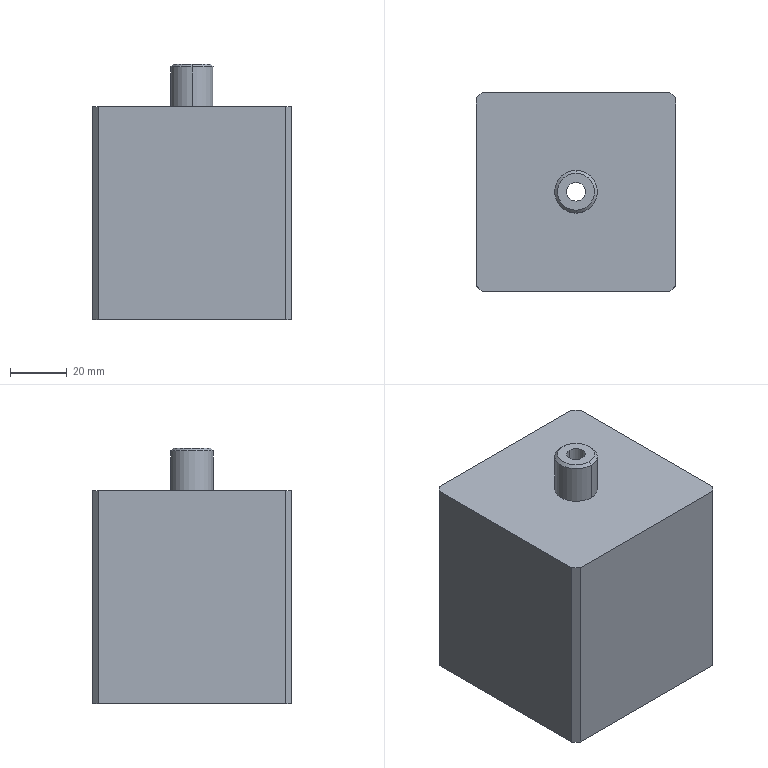NC program | NX | posted with a generic post | part box 70 x 70 x 90 mm
Lines 107 to 966 of 10206:
(ZLEVEL_PROFILE_COPY_1_COPY , TOOL : D16)
N212 T22 M6
N214 G54
N216 G17 G0 G90 X-6.657 Y-6.984 S7500 M3
N218 G43 Z30. H22
N220 Z1.4
N222 G94 G1 X-5.215 Y-7.622 Z1.317 F1000.
N224 X-2.644 Y-8.278 Z1.178
N226 X0. Y-8.499 Z1.039
N228 X2.644 Y-8.278 Z0.9
N230 X5.215 Y-7.622 Z0.761
N232 X7.642 Y-6.548 Z0.622
N234 X8.469 Y-6.028 Z0.571
N236 Y6.028 Z-0.061
N238 X7.642 Y6.548 Z-0.112
N240 X5.215 Y7.622 Z-0.251
N242 X2.644 Y8.278 Z-0.39
N244 X0. Y8.499 Z-0.529
N246 X-2.644 Y8.278 Z-0.668
N248 X-5.215 Y7.622 Z-0.808
N250 X-7.642 Y6.548 Z-0.947
N252 X-8.469 Y6.028 Z-0.998
N254 Y-6.028 F2500.
N256 G3 X8.469 Y-6.028 R15.91
N258 G1 Y6.028
N260 G3 X-8.469 Y6.028 R15.91
N262 G1 X-8.461 Y5.368 Z-1.013
N264 X-8.452 Y4.709 Z-1.028
N266 X-8.444 Y4.049 Z-1.043
N268 X-8.436 Y3.389 Z-1.058
N270 X-8.428 Y2.73 Z-1.073
N272 X-8.42 Y2.07 Z-1.089
N274 X-8.412 Y1.411 Z-1.104
N276 X-8.405 Y0.751 Z-1.119
N278 X-8.397 Y0.092 Z-1.134
N280 X-8.39 Y-0.568 Z-1.149
N282 X-8.383 Y-1.228 Z-1.164
N284 X-8.376 Y-1.887 Z-1.179
N286 X-8.369 Y-2.547 Z-1.194
N288 X-8.363 Y-3.206 Z-1.209
N290 X-8.356 Y-3.866 Z-1.225
N292 X-8.35 Y-4.525 Z-1.24
N294 X-8.344 Y-5.185 Z-1.255
N296 X-8.338 Y-5.845 Z-1.27
N298 X-8.337 Y-5.954 Z-1.273
N300 X-7.992 Y-6.158 Z-1.283
N302 X-7.42 Y-6.472 Z-1.3
N304 X-6.834 Y-6.762 Z-1.315
N306 X-6.238 Y-7.028 Z-1.33
N308 X-5.631 Y-7.269 Z-1.346
N310 X-5.014 Y-7.485 Z-1.361
N312 X-4.39 Y-7.675 Z-1.376
N314 X-3.759 Y-7.84 Z-1.391
N316 X-3.121 Y-7.977 Z-1.406
N318 X-2.479 Y-8.089 Z-1.421
N320 X-1.833 Y-8.174 Z-1.436
N322 X-1.184 Y-8.232 Z-1.451
N324 X-0.533 Y-8.263 Z-1.466
N326 X0.118 Y-8.268 Z-1.482
N328 X0.769 Y-8.246 Z-1.497
N330 X1.418 Y-8.196 Z-1.512
N332 X2.065 Y-8.12 Z-1.527
N334 X2.707 Y-8.018 Z-1.542
N336 X3.345 Y-7.889 Z-1.557
N338 X3.976 Y-7.734 Z-1.572
N340 X4.601 Y-7.553 Z-1.587
N342 X5.217 Y-7.346 Z-1.603
N344 X5.824 Y-7.115 Z-1.618
N346 X6.422 Y-6.858 Z-1.633
N348 X7.403 Y-6.371 Z-1.658
N350 X7.581 Y-6.272 Z-1.663
N352 X8.203 Y-5.906 Z-1.684
N354 X8.224 Y-5.605 Z-1.693
N356 X8.221 Y-4.945 Z-1.708
N358 X8.219 Y-4.285 Z-1.723
N360 X8.217 Y-3.626 Z-1.739
N362 X8.215 Y-2.966 Z-1.754
N364 X8.213 Y-2.307 Z-1.769
N366 X8.212 Y-1.647 Z-1.784
N368 X8.21 Y-0.988 Z-1.799
N370 X8.209 Y-0.328 Z-1.814
N372 X8.207 Y0.331 Z-1.829
N374 X8.206 Y0.991 Z-1.844
N376 X8.205 Y1.651 Z-1.86
N378 X8.204 Y2.31 Z-1.875
N380 X8.203 Y2.97 Z-1.89
N382 X8.202 Y3.629 Z-1.905
N384 Y4.289 Z-1.92
N386 X8.201 Y4.948 Z-1.935
N388 X8.197 Y5.881 Z-1.963
N390 X7.564 Y6.249 Z-1.98
N392 X6.991 Y6.551 Z-1.996
N394 G3 X-8.203 Y5.876 R15.64
N396 G1 X-8.2 Y5.216 Z-2.011
N398 Y4.557 Z-2.026
N400 Y-4.676 Z-2.237
N402 X-8.195 Y-5.881 Z-2.265
N404 X-8.1 Y-5.939 Z-2.268
N406 X-7.529 Y-6.269 Z-2.283
N408 X-6.944 Y-6.574 Z-2.298
N410 X-6.347 Y-6.854 Z-2.313
N412 X-5.739 Y-7.109 Z-2.328
N414 X-5.12 Y-7.338 Z-2.343
N416 X-4.493 Y-7.541 Z-2.358
N418 X-3.857 Y-7.717 Z-2.374
N420 X-3.215 Y-7.866 Z-2.389
N422 X-2.567 Y-7.988 Z-2.404
N424 X-1.914 Y-8.082 Z-2.419
N426 X-1.258 Y-8.149 Z-2.434
N428 X-0.6 Y-8.188 Z-2.449
N430 X0.06 Y-8.2 Z-2.464
N432 X0.719 Y-8.183 Z-2.479
N434 X1.377 Y-8.139 Z-2.494
N436 X2.032 Y-8.067 Z-2.51
N438 X2.684 Y-7.968 Z-2.525
N440 X3.332 Y-7.841 Z-2.54
N442 X3.973 Y-7.687 Z-2.555
N444 X4.607 Y-7.506 Z-2.57
N446 X5.233 Y-7.299 Z-2.585
N448 X5.85 Y-7.065 Z-2.6
N450 X6.456 Y-6.805 Z-2.615
N452 X7.051 Y-6.521 Z-2.631
N454 X8.126 Y-5.924 Z-2.659
N456 X8.2 Y-5.876 Z-2.661
N458 Y-5.217 Z-2.676
N460 Y4.676 Z-2.903
N462 X8.196 Y5.882 Z-2.93
N464 X8.101 Y5.938 Z-2.933
N466 X7.53 Y6.268 Z-2.948
N468 X6.946 Y6.573 Z-2.963
N470 X6.349 Y6.853 Z-2.978
N472 X5.741 Y7.108 Z-2.993
N474 G3 X-8.2 Y5.878 R15.64
N476 G1 Y5.876
N478 Y-4.676 Z-3.235
N480 X-8.195 Y-5.881 Z-3.263
N482 X-8.1 Y-5.939 Z-3.266
N484 X-7.529 Y-6.269 Z-3.281
N486 X-6.944 Y-6.574 Z-3.296
N488 X-6.347 Y-6.854 Z-3.311
N490 X-5.739 Y-7.109 Z-3.326
N492 X-5.12 Y-7.338 Z-3.341
N494 X-4.493 Y-7.541 Z-3.356
N496 X-3.857 Y-7.717 Z-3.371
N498 X-3.215 Y-7.866 Z-3.386
N500 X-2.567 Y-7.988 Z-3.402
N502 X-1.914 Y-8.082 Z-3.417
N504 X-1.258 Y-8.149 Z-3.432
N506 X-0.6 Y-8.188 Z-3.447
N508 X0.06 Y-8.2 Z-3.462
N510 X0.719 Y-8.183 Z-3.477
N512 X1.377 Y-8.139 Z-3.492
N514 X2.032 Y-8.067 Z-3.507
N516 X2.684 Y-7.968 Z-3.523
N518 X3.332 Y-7.841 Z-3.538
N520 X3.973 Y-7.687 Z-3.553
N522 X4.607 Y-7.506 Z-3.568
N524 X5.233 Y-7.299 Z-3.583
N526 X5.85 Y-7.065 Z-3.598
N528 X6.456 Y-6.805 Z-3.613
N530 X7.051 Y-6.521 Z-3.628
N532 X8.126 Y-5.924 Z-3.656
N534 X8.2 Y-5.876 Z-3.659
N536 Y-5.217 Z-3.674
N538 Y4.676 Z-3.9
N540 X8.196 Y5.882 Z-3.928
N542 X8.1 Y5.939 Z-3.931
N544 X7.529 Y6.269 Z-3.946
N546 X6.944 Y6.574 Z-3.961
N548 X6.347 Y6.854 Z-3.976
N550 X5.739 Y7.109 Z-3.991
N552 G3 X-8.2 Y5.878 R15.64
N554 G1 Y5.876
N556 Y-4.676 Z-4.233
N558 X-8.195 Y-5.881 Z-4.261
N560 X-8.1 Y-5.939 Z-4.263
N562 X-7.529 Y-6.269 Z-4.278
N564 X-6.944 Y-6.574 Z-4.294
N566 X-6.347 Y-6.854 Z-4.309
N568 X-5.739 Y-7.109 Z-4.324
N570 X-5.12 Y-7.338 Z-4.339
N572 X-4.493 Y-7.541 Z-4.354
N574 X-3.857 Y-7.717 Z-4.369
N576 X-3.215 Y-7.866 Z-4.384
N578 X-2.567 Y-7.988 Z-4.399
N580 X-1.914 Y-8.082 Z-4.414
N582 X-1.258 Y-8.149 Z-4.43
N584 X-0.6 Y-8.188 Z-4.445
N586 X0.06 Y-8.2 Z-4.46
N588 X0.719 Y-8.183 Z-4.475
N590 X1.377 Y-8.139 Z-4.49
N592 X2.032 Y-8.067 Z-4.505
N594 X2.684 Y-7.968 Z-4.52
N596 X3.332 Y-7.841 Z-4.535
N598 X3.973 Y-7.687 Z-4.551
N600 X4.607 Y-7.506 Z-4.566
N602 X5.233 Y-7.299 Z-4.581
N604 X5.85 Y-7.065 Z-4.596
N606 X6.456 Y-6.805 Z-4.611
N608 X7.051 Y-6.521 Z-4.626
N610 X8.126 Y-5.924 Z-4.654
N612 X8.2 Y-5.876 Z-4.656
N614 Y-5.217 Z-4.671
N616 Y4.676 Z-4.898
N618 X8.196 Y5.882 Z-4.926
N620 X8.1 Y5.939 Z-4.928
N622 X7.529 Y6.269 Z-4.944
N624 X6.944 Y6.574 Z-4.959
N626 X6.347 Y6.854 Z-4.974
N628 X5.739 Y7.109 Z-4.989
N630 G3 X-8.2 Y5.878 R15.64
N632 G1 Y5.876
N634 Y-4.676 Z-5.231
N636 X-8.195 Y-5.881 Z-5.258
N638 X-8.1 Y-5.939 Z-5.261
N640 X-7.529 Y-6.269 Z-5.276
N642 X-6.944 Y-6.574 Z-5.291
N644 X-6.347 Y-6.854 Z-5.306
N646 X-5.739 Y-7.109 Z-5.322
N648 X-5.12 Y-7.338 Z-5.337
N650 X-4.493 Y-7.541 Z-5.352
N652 X-3.857 Y-7.717 Z-5.367
N654 X-3.215 Y-7.866 Z-5.382
N656 X-2.567 Y-7.988 Z-5.397
N658 X-1.914 Y-8.082 Z-5.412
N660 X-1.258 Y-8.149 Z-5.427
N662 X-0.6 Y-8.188 Z-5.443
N664 X0.06 Y-8.2 Z-5.458
N666 X0.719 Y-8.183 Z-5.473
N668 X1.377 Y-8.139 Z-5.488
N670 X2.032 Y-8.067 Z-5.503
N672 X2.684 Y-7.968 Z-5.518
N674 X3.332 Y-7.841 Z-5.533
N676 X3.973 Y-7.687 Z-5.548
N678 X4.607 Y-7.506 Z-5.563
N680 X5.233 Y-7.299 Z-5.579
N682 X5.85 Y-7.065 Z-5.594
N684 X6.456 Y-6.805 Z-5.609
N686 X7.051 Y-6.521 Z-5.624
N688 X8.126 Y-5.924 Z-5.652
N690 X8.2 Y-5.876 Z-5.654
N692 Y-5.217 Z-5.669
N694 Y4.676 Z-5.896
N696 X8.196 Y5.882 Z-5.924
N698 X8.1 Y5.939 Z-5.926
N700 X7.529 Y6.269 Z-5.941
N702 X6.944 Y6.574 Z-5.957
N704 X6.347 Y6.854 Z-5.972
N706 X5.739 Y7.109 Z-5.987
N708 G3 X-8.2 Y5.878 R15.64
N710 G1 Y5.876
N712 Y-4.676 Z-6.229
N714 X-8.195 Y-5.881 Z-6.256
N716 X-8.1 Y-5.939 Z-6.259
N718 X-7.529 Y-6.269 Z-6.274
N720 X-6.944 Y-6.574 Z-6.289
N722 X-6.347 Y-6.854 Z-6.304
N724 X-5.739 Y-7.109 Z-6.319
N726 X-5.12 Y-7.338 Z-6.334
N728 X-4.493 Y-7.541 Z-6.35
N730 X-3.857 Y-7.717 Z-6.365
N732 X-3.215 Y-7.866 Z-6.38
N734 X-2.567 Y-7.988 Z-6.395
N736 X-1.914 Y-8.082 Z-6.41
N738 X-1.258 Y-8.149 Z-6.425
N740 X-0.6 Y-8.188 Z-6.44
N742 X0.06 Y-8.2 Z-6.455
N744 X0.719 Y-8.183 Z-6.471
N746 X1.377 Y-8.139 Z-6.486
N748 X2.032 Y-8.067 Z-6.501
N750 X2.684 Y-7.968 Z-6.516
N752 X3.332 Y-7.841 Z-6.531
N754 X3.973 Y-7.687 Z-6.546
N756 X4.607 Y-7.506 Z-6.561
N758 X5.233 Y-7.299 Z-6.576
N760 X5.85 Y-7.065 Z-6.591
N762 X6.456 Y-6.805 Z-6.607
N764 X7.051 Y-6.521 Z-6.622
N766 X8.126 Y-5.924 Z-6.65
N768 X8.2 Y-5.876 Z-6.652
N770 Y-5.217 Z-6.667
N772 Y4.676 Z-6.894
N774 X8.195 Y5.882 Z-6.921
N776 X8.1 Y5.939 Z-6.924
N778 X7.529 Y6.269 Z-6.939
N780 X6.944 Y6.574 Z-6.954
N782 X6.347 Y6.854 Z-6.969
N784 X5.739 Y7.109 Z-6.985
N786 G3 X-8.2 Y5.878 R15.64
N788 G1 Y5.876
N790 Y-4.676 Z-7.226
N792 X-8.195 Y-5.881 Z-7.254
N794 X-8.1 Y-5.939 Z-7.257
N796 X-7.529 Y-6.269 Z-7.272
N798 X-6.944 Y-6.574 Z-7.287
N800 X-6.347 Y-6.854 Z-7.302
N802 X-5.739 Y-7.109 Z-7.317
N804 X-5.12 Y-7.338 Z-7.332
N806 X-4.493 Y-7.541 Z-7.347
N808 X-3.857 Y-7.717 Z-7.363
N810 X-3.215 Y-7.866 Z-7.378
N812 X-2.567 Y-7.988 Z-7.393
N814 X-1.914 Y-8.082 Z-7.408
N816 X-1.258 Y-8.149 Z-7.423
N818 X-0.6 Y-8.188 Z-7.438
N820 X0.06 Y-8.2 Z-7.453
N822 X0.719 Y-8.183 Z-7.468
N824 X1.377 Y-8.139 Z-7.483
N826 X2.032 Y-8.067 Z-7.499
N828 X2.684 Y-7.968 Z-7.514
N830 X3.332 Y-7.841 Z-7.529
N832 X3.973 Y-7.687 Z-7.544
N834 X4.607 Y-7.506 Z-7.559
N836 X5.233 Y-7.299 Z-7.574
N838 X5.85 Y-7.065 Z-7.589
N840 X6.456 Y-6.805 Z-7.604
N842 X7.051 Y-6.521 Z-7.62
N844 X8.126 Y-5.924 Z-7.648
N846 X8.2 Y-5.876 Z-7.65
N848 Y-5.217 Z-7.665
N850 Y4.676 Z-7.892
N852 X8.195 Y5.882 Z-7.919
N854 X8.1 Y5.939 Z-7.922
N856 X7.529 Y6.269 Z-7.937
N858 X6.944 Y6.574 Z-7.952
N860 X6.347 Y6.854 Z-7.967
N862 X5.739 Y7.109 Z-7.982
N864 G3 X-8.2 Y5.878 R15.64
N866 G1 Y5.876
N868 Y-4.676 Z-8.224
N870 X-8.195 Y-5.881 Z-8.252
N872 X-8.1 Y-5.939 Z-8.254
N874 X-7.529 Y-6.269 Z-8.27
N876 X-6.944 Y-6.574 Z-8.285
N878 X-6.347 Y-6.854 Z-8.3
N880 X-5.739 Y-7.109 Z-8.315
N882 X-5.12 Y-7.338 Z-8.33
N884 X-4.493 Y-7.541 Z-8.345
N886 X-3.857 Y-7.717 Z-8.36
N888 X-3.215 Y-7.866 Z-8.375
N890 X-2.567 Y-7.988 Z-8.391
N892 X-1.914 Y-8.082 Z-8.406
N894 X-1.258 Y-8.149 Z-8.421
N896 X-0.6 Y-8.188 Z-8.436
N898 X0.06 Y-8.2 Z-8.451
N900 X0.719 Y-8.183 Z-8.466
N902 X1.377 Y-8.139 Z-8.481
N904 X2.032 Y-8.067 Z-8.496
N906 X2.684 Y-7.968 Z-8.511
N908 X3.332 Y-7.841 Z-8.527
N910 X3.973 Y-7.687 Z-8.542
N912 X4.607 Y-7.506 Z-8.557
N914 X5.233 Y-7.299 Z-8.572
N916 X5.85 Y-7.065 Z-8.587
N918 X6.456 Y-6.805 Z-8.602
N920 X7.051 Y-6.521 Z-8.617
N922 X8.126 Y-5.924 Z-8.645
N924 X8.2 Y-5.876 Z-8.648
N926 Y-5.217 Z-8.663
N928 Y4.676 Z-8.889
N930 X8.195 Y5.882 Z-8.917
N932 X8.1 Y5.939 Z-8.92
N934 X7.529 Y6.269 Z-8.935
N936 X6.944 Y6.574 Z-8.95
N938 X6.347 Y6.854 Z-8.965
N940 X5.739 Y7.109 Z-8.98
N942 G3 X-8.2 Y5.878 R15.64
N944 G1 Y5.876
N946 Y-4.676 Z-9.222
N948 X-8.195 Y-5.881 Z-9.25
N950 X-8.1 Y-5.939 Z-9.252
N952 X-7.529 Y-6.269 Z-9.267
N954 X-6.944 Y-6.574 Z-9.283
N956 X-6.347 Y-6.854 Z-9.298
N958 X-5.739 Y-7.109 Z-9.313
N960 X-5.12 Y-7.338 Z-9.328
N962 X-4.493 Y-7.541 Z-9.343
N964 X-3.857 Y-7.717 Z-9.358
N966 X-3.215 Y-7.866 Z-9.373
N968 X-2.567 Y-7.988 Z-9.388
N970 X-1.914 Y-8.082 Z-9.403
N972 X-1.258 Y-8.149 Z-9.419
N974 X-0.6 Y-8.188 Z-9.434
N976 X0.06 Y-8.2 Z-9.449
N978 X0.719 Y-8.183 Z-9.464
N980 X1.377 Y-8.139 Z-9.479
N982 X2.032 Y-8.067 Z-9.494
N984 X2.684 Y-7.968 Z-9.509
N986 X3.332 Y-7.841 Z-9.524
N988 X3.973 Y-7.687 Z-9.54
N990 X4.607 Y-7.506 Z-9.555
N992 X5.233 Y-7.299 Z-9.57
N994 X5.85 Y-7.065 Z-9.585
N996 X6.456 Y-6.805 Z-9.6
N998 X7.051 Y-6.521 Z-9.615
N1000 X8.126 Y-5.924 Z-9.643
N1002 X8.2 Y-5.876 Z-9.645
N1004 Y-5.217 Z-9.66
N1006 Y4.676 Z-9.887
N1008 X8.195 Y5.882 Z-9.915
N1010 X8.1 Y5.939 Z-9.917
N1012 X7.529 Y6.269 Z-9.933
N1014 X6.944 Y6.574 Z-9.948
N1016 X6.347 Y6.854 Z-9.963
N1018 X5.739 Y7.109 Z-9.978
N1020 G3 X-8.2 Y5.878 R15.64
N1022 G1 Y5.876
N1024 Y-4.676 Z-10.22
N1026 X-8.195 Y-5.881 Z-10.247
N1028 X-8.1 Y-5.939 Z-10.25
N1030 X-7.529 Y-6.269 Z-10.265
N1032 X-6.944 Y-6.574 Z-10.28
N1034 X-6.347 Y-6.854 Z-10.295
N1036 X-5.739 Y-7.109 Z-10.311
N1038 X-5.12 Y-7.338 Z-10.326
N1040 X-4.493 Y-7.541 Z-10.341
N1042 X-3.857 Y-7.717 Z-10.356
N1044 X-3.215 Y-7.866 Z-10.371
N1046 X-2.567 Y-7.988 Z-10.386
N1048 X-1.914 Y-8.082 Z-10.401
N1050 X-1.258 Y-8.149 Z-10.416
N1052 X-0.6 Y-8.188 Z-10.431
N1054 X0.06 Y-8.2 Z-10.447
N1056 X0.719 Y-8.183 Z-10.462
N1058 X1.377 Y-8.139 Z-10.477
N1060 X2.032 Y-8.067 Z-10.492
N1062 X2.684 Y-7.968 Z-10.507
N1064 X3.332 Y-7.841 Z-10.522
N1066 X3.973 Y-7.687 Z-10.537
N1068 X4.607 Y-7.506 Z-10.552
N1070 X5.233 Y-7.299 Z-10.568
N1072 X5.85 Y-7.065 Z-10.583
N1074 X6.456 Y-6.805 Z-10.598
N1076 X7.051 Y-6.521 Z-10.613
N1078 X8.126 Y-5.924 Z-10.641
N1080 X8.2 Y-5.876 Z-10.643
N1082 Y-5.217 Z-10.658
N1084 Y4.676 Z-10.885
N1086 X8.195 Y5.882 Z-10.913
N1088 X8.1 Y5.939 Z-10.915
N1090 X7.529 Y6.269 Z-10.93
N1092 X6.944 Y6.574 Z-10.946
N1094 X6.347 Y6.854 Z-10.961
N1096 X5.739 Y7.109 Z-10.976
N1098 G3 X-8.2 Y5.878 R15.64
N1100 G1 Y5.876
N1102 Y-4.676 Z-11.218
N1104 X-8.195 Y-5.881 Z-11.245
N1106 X-8.1 Y-5.939 Z-11.248
N1108 X-7.529 Y-6.269 Z-11.263
N1110 X-6.944 Y-6.574 Z-11.278
N1112 X-6.347 Y-6.854 Z-11.293
N1114 X-5.739 Y-7.109 Z-11.308
N1116 X-5.12 Y-7.338 Z-11.323
N1118 X-4.493 Y-7.541 Z-11.339
N1120 X-3.857 Y-7.717 Z-11.354
N1122 X-3.215 Y-7.866 Z-11.369
N1124 X-2.567 Y-7.988 Z-11.384
N1126 X-1.914 Y-8.082 Z-11.399
N1128 X-1.258 Y-8.149 Z-11.414
N1130 X-0.6 Y-8.188 Z-11.429
N1132 X0.06 Y-8.2 Z-11.444
N1134 X0.719 Y-8.183 Z-11.46
N1136 X1.377 Y-8.139 Z-11.475
N1138 X2.032 Y-8.067 Z-11.49
N1140 X2.684 Y-7.968 Z-11.505
N1142 X3.332 Y-7.841 Z-11.52
N1144 X3.973 Y-7.687 Z-11.535
N1146 X4.607 Y-7.506 Z-11.55
N1148 X5.233 Y-7.299 Z-11.565
N1150 X5.85 Y-7.065 Z-11.58
N1152 X6.456 Y-6.805 Z-11.596
N1154 X7.051 Y-6.521 Z-11.611
N1156 X8.126 Y-5.924 Z-11.639
N1158 X8.2 Y-5.876 Z-11.641
N1160 Y-5.217 Z-11.656
N1162 Y4.676 Z-11.883
N1164 X8.195 Y5.881 Z-11.91
N1166 X8.1 Y5.939 Z-11.913
N1168 X7.529 Y6.269 Z-11.928
N1170 X6.944 Y6.574 Z-11.943
N1172 X6.347 Y6.854 Z-11.958
N1174 X5.739 Y7.109 Z-11.974
N1176 G3 X-8.2 Y5.878 R15.64
N1178 G1 Y5.876
N1180 Y-4.676 Z-12.215
N1182 X-8.195 Y-5.881 Z-12.243
N1184 X-8.1 Y-5.939 Z-12.246
N1186 X-7.529 Y-6.269 Z-12.261
N1188 X-6.944 Y-6.574 Z-12.276
N1190 X-6.347 Y-6.854 Z-12.291
N1192 X-5.739 Y-7.109 Z-12.306
N1194 X-5.12 Y-7.338 Z-12.321
N1196 X-4.493 Y-7.541 Z-12.336
N1198 X-3.857 Y-7.717 Z-12.351
N1200 X-3.215 Y-7.866 Z-12.367
N1202 X-2.567 Y-7.988 Z-12.382
N1204 X-1.914 Y-8.082 Z-12.397
N1206 X-1.258 Y-8.149 Z-12.412
N1208 X-0.6 Y-8.188 Z-12.427
N1210 X0.06 Y-8.2 Z-12.442
N1212 X0.719 Y-8.183 Z-12.457
N1214 X1.377 Y-8.139 Z-12.472
N1216 X2.032 Y-8.067 Z-12.488
N1218 X2.684 Y-7.968 Z-12.503
N1220 X3.332 Y-7.841 Z-12.518
N1222 X3.973 Y-7.687 Z-12.533
N1224 X4.607 Y-7.506 Z-12.548
N1226 X5.233 Y-7.299 Z-12.563
N1228 X5.85 Y-7.065 Z-12.578
N1230 X6.456 Y-6.805 Z-12.593
N1232 X7.051 Y-6.521 Z-12.608
N1234 X8.126 Y-5.924 Z-12.637
N1236 X8.2 Y-5.876 Z-12.639
N1238 Y-5.217 Z-12.654
N1240 Y4.676 Z-12.881
N1242 X8.195 Y5.881 Z-12.908
N1244 X8.1 Y5.939 Z-12.911
N1246 X7.529 Y6.269 Z-12.926
N1248 X6.944 Y6.574 Z-12.941
N1250 X6.347 Y6.854 Z-12.956
N1252 X5.739 Y7.109 Z-12.971
N1254 G3 X-8.2 Y5.878 R15.64
N1256 G1 Y5.876
N1258 Y-4.676 Z-13.213
N1260 X-8.195 Y-5.881 Z-13.241
N1262 X-8.1 Y-5.939 Z-13.243
N1264 X-7.529 Y-6.269 Z-13.259
N1266 X-6.944 Y-6.574 Z-13.274
N1268 X-6.347 Y-6.854 Z-13.289
N1270 X-5.739 Y-7.109 Z-13.304
N1272 X-5.12 Y-7.338 Z-13.319
N1274 X-4.493 Y-7.541 Z-13.334
N1276 X-3.857 Y-7.717 Z-13.349
N1278 X-3.215 Y-7.866 Z-13.364
N1280 X-2.567 Y-7.988 Z-13.38
N1282 X-1.914 Y-8.082 Z-13.395
N1284 X-1.258 Y-8.149 Z-13.41
N1286 X-0.6 Y-8.188 Z-13.425
N1288 X0.06 Y-8.2 Z-13.44
N1290 X0.719 Y-8.183 Z-13.455
N1292 X1.377 Y-8.139 Z-13.47
N1294 X2.032 Y-8.067 Z-13.485
N1296 X2.684 Y-7.968 Z-13.5
N1298 X3.332 Y-7.841 Z-13.516
N1300 X3.973 Y-7.687 Z-13.531
N1302 X4.607 Y-7.506 Z-13.546
N1304 X5.233 Y-7.299 Z-13.561
N1306 X5.85 Y-7.065 Z-13.576
N1308 X6.456 Y-6.805 Z-13.591
N1310 X7.051 Y-6.521 Z-13.606
N1312 X8.126 Y-5.924 Z-13.634
N1314 X8.2 Y-5.876 Z-13.637
N1316 Y-5.217 Z-13.652
N1318 Y4.676 Z-13.878
N1320 X8.195 Y5.881 Z-13.906
N1322 X8.1 Y5.939 Z-13.909
N1324 X7.529 Y6.269 Z-13.924
N1326 X6.944 Y6.574 Z-13.939
N1328 X6.347 Y6.854 Z-13.954
N1330 X5.739 Y7.109 Z-13.969
N1332 G3 X-8.2 Y5.878 R15.64
N1334 G1 Y5.876
N1336 Y-4.676 Z-14.211
N1338 X-8.195 Y-5.881 Z-14.239
N1340 X-8.1 Y-5.939 Z-14.241
N1342 X-7.529 Y-6.269 Z-14.256
N1344 X-6.944 Y-6.574 Z-14.271
N1346 X-6.347 Y-6.854 Z-14.287
N1348 X-5.739 Y-7.109 Z-14.302
N1350 X-5.12 Y-7.338 Z-14.317
N1352 X-4.493 Y-7.541 Z-14.332
N1354 X-3.857 Y-7.717 Z-14.347
N1356 X-3.215 Y-7.866 Z-14.362
N1358 X-2.567 Y-7.988 Z-14.377
N1360 X-1.914 Y-8.082 Z-14.392
N1362 X-1.258 Y-8.149 Z-14.408
N1364 X-0.6 Y-8.188 Z-14.423
N1366 X0.06 Y-8.2 Z-14.438
N1368 X0.719 Y-8.183 Z-14.453
N1370 X1.377 Y-8.139 Z-14.468
N1372 X2.032 Y-8.067 Z-14.483
N1374 X2.684 Y-7.968 Z-14.498
N1376 X3.332 Y-7.841 Z-14.513
N1378 X3.973 Y-7.687 Z-14.528
N1380 X4.607 Y-7.506 Z-14.544
N1382 X5.233 Y-7.299 Z-14.559
N1384 X5.85 Y-7.065 Z-14.574
N1386 X6.456 Y-6.805 Z-14.589
N1388 X7.051 Y-6.521 Z-14.604
N1390 X8.126 Y-5.924 Z-14.632
N1392 X8.2 Y-5.876 Z-14.634
N1394 Y-5.217 Z-14.649
N1396 Y4.676 Z-14.876
N1398 X8.195 Y5.881 Z-14.904
N1400 X8.1 Y5.939 Z-14.906
N1402 X7.529 Y6.269 Z-14.922
N1404 X6.944 Y6.574 Z-14.937
N1406 X6.347 Y6.854 Z-14.952
N1408 X5.739 Y7.109 Z-14.967
N1410 G3 X-8.2 Y5.878 R15.64
N1412 G1 Y5.876
N1414 Y-4.676 Z-15.209
N1416 X-8.195 Y-5.881 Z-15.236
N1418 X-8.1 Y-5.939 Z-15.239
N1420 X-7.529 Y-6.269 Z-15.254
N1422 X-6.944 Y-6.574 Z-15.269
N1424 X-6.347 Y-6.854 Z-15.284
N1426 X-5.739 Y-7.109 Z-15.3
N1428 X-5.12 Y-7.338 Z-15.315
N1430 X-4.493 Y-7.541 Z-15.33
N1432 X-3.857 Y-7.717 Z-15.345
N1434 X-3.215 Y-7.866 Z-15.36
N1436 X-2.567 Y-7.988 Z-15.375
N1438 X-1.914 Y-8.082 Z-15.39
N1440 X-1.258 Y-8.149 Z-15.405
N1442 X-0.6 Y-8.188 Z-15.42
N1444 X0.06 Y-8.2 Z-15.436
N1446 X0.719 Y-8.183 Z-15.451
N1448 X1.377 Y-8.139 Z-15.466
N1450 X2.032 Y-8.067 Z-15.481
N1452 X2.684 Y-7.968 Z-15.496
N1454 X3.332 Y-7.841 Z-15.511
N1456 X3.973 Y-7.687 Z-15.526
N1458 X4.607 Y-7.506 Z-15.541
N1460 X5.233 Y-7.299 Z-15.557
N1462 X5.85 Y-7.065 Z-15.572
N1464 X6.456 Y-6.805 Z-15.587
N1466 X7.051 Y-6.521 Z-15.602
N1468 X8.126 Y-5.924 Z-15.63
N1470 X8.2 Y-5.876 Z-15.632
N1472 Y-5.217 Z-15.647
N1474 Y4.676 Z-15.874
N1476 X8.195 Y5.881 Z-15.902
N1478 X8.1 Y5.939 Z-15.904
N1480 X7.529 Y6.269 Z-15.919
N1482 X6.944 Y6.574 Z-15.934
N1484 X6.347 Y6.854 Z-15.95
N1486 X5.739 Y7.109 Z-15.965
N1488 G3 X-8.2 Y5.878 R15.64
N1490 G1 Y5.876
N1492 Y-4.676 Z-16.207
N1494 X-8.195 Y-5.881 Z-16.234
N1496 X-8.1 Y-5.939 Z-16.237
N1498 X-7.529 Y-6.269 Z-16.252
N1500 X-6.944 Y-6.574 Z-16.267
N1502 X-6.347 Y-6.854 Z-16.282
N1504 X-5.739 Y-7.109 Z-16.297
N1506 X-5.12 Y-7.338 Z-16.312
N1508 X-4.493 Y-7.541 Z-16.328
N1510 X-3.857 Y-7.717 Z-16.343
N1512 X-3.215 Y-7.866 Z-16.358
N1514 X-2.567 Y-7.988 Z-16.373
N1516 X-1.914 Y-8.082 Z-16.388
N1518 X-1.258 Y-8.149 Z-16.403
N1520 X-0.6 Y-8.188 Z-16.418
N1522 X0.06 Y-8.2 Z-16.433
N1524 X0.719 Y-8.183 Z-16.448
N1526 X1.377 Y-8.139 Z-16.464
N1528 X2.032 Y-8.067 Z-16.479
N1530 X2.684 Y-7.968 Z-16.494
N1532 X3.332 Y-7.841 Z-16.509
N1534 X3.973 Y-7.687 Z-16.524
N1536 X4.607 Y-7.506 Z-16.539
N1538 X5.233 Y-7.299 Z-16.554
N1540 X5.85 Y-7.065 Z-16.569
N1542 X6.456 Y-6.805 Z-16.585
N1544 X7.051 Y-6.521 Z-16.6
N1546 X8.126 Y-5.924 Z-16.628
N1548 X8.2 Y-5.876 Z-16.63
N1550 Y-5.217 Z-16.645
N1552 Y4.676 Z-16.872
N1554 X8.195 Y5.881 Z-16.899
N1556 X8.1 Y5.939 Z-16.902
N1558 X7.529 Y6.269 Z-16.917
N1560 X6.944 Y6.574 Z-16.932
N1562 X6.347 Y6.854 Z-16.947
N1564 X5.739 Y7.109 Z-16.963
N1566 G3 X-8.2 Y5.878 R15.64
N1568 G1 Y5.876
N1570 Y-4.676 Z-17.204
N1572 X-8.195 Y-5.881 Z-17.232
N1574 X-8.1 Y-5.939 Z-17.235
N1576 X-7.529 Y-6.269 Z-17.25
N1578 X-6.944 Y-6.574 Z-17.265
N1580 X-6.347 Y-6.854 Z-17.28
N1582 X-5.739 Y-7.109 Z-17.295
N1584 X-5.12 Y-7.338 Z-17.31
N1586 X-4.493 Y-7.541 Z-17.325
N1588 X-3.857 Y-7.717 Z-17.34
N1590 X-3.215 Y-7.866 Z-17.356
N1592 X-2.567 Y-7.988 Z-17.371
N1594 X-1.914 Y-8.082 Z-17.386
N1596 X-1.258 Y-8.149 Z-17.401
N1598 X-0.6 Y-8.188 Z-17.416
N1600 X0.06 Y-8.2 Z-17.431
N1602 X0.719 Y-8.183 Z-17.446
N1604 X1.377 Y-8.139 Z-17.461
N1606 X2.032 Y-8.067 Z-17.477
N1608 X2.684 Y-7.968 Z-17.492
N1610 X3.332 Y-7.841 Z-17.507
N1612 X3.973 Y-7.687 Z-17.522
N1614 X4.607 Y-7.506 Z-17.537
N1616 X5.233 Y-7.299 Z-17.552
N1618 X5.85 Y-7.065 Z-17.567
N1620 X6.456 Y-6.805 Z-17.582
N1622 X7.051 Y-6.521 Z-17.597
N1624 X8.126 Y-5.924 Z-17.626
N1626 X8.2 Y-5.876 Z-17.628
N1628 Y-5.217 Z-17.643
N1630 Y4.676 Z-17.87
N1632 X8.195 Y5.881 Z-17.897
N1634 X8.1 Y5.939 Z-17.9
N1636 X7.529 Y6.269 Z-17.915
N1638 X6.944 Y6.574 Z-17.93
N1640 X6.347 Y6.854 Z-17.945
N1642 X5.739 Y7.109 Z-17.96
N1644 G3 X-8.2 Y5.878 R15.64
N1646 G1 Y5.876
N1648 Y-4.676 Z-18.202
N1650 X-8.195 Y-5.881 Z-18.23
N1652 X-8.1 Y-5.939 Z-18.232
N1654 X-7.529 Y-6.269 Z-18.248
N1656 X-6.944 Y-6.574 Z-18.263
N1658 X-6.347 Y-6.854 Z-18.278
N1660 X-5.739 Y-7.109 Z-18.293
N1662 X-5.12 Y-7.338 Z-18.308
N1664 X-4.493 Y-7.541 Z-18.323
N1666 X-3.857 Y-7.717 Z-18.338
N1668 X-3.215 Y-7.866 Z-18.353
N1670 X-2.567 Y-7.988 Z-18.368
N1672 X-1.914 Y-8.082 Z-18.384
N1674 X-1.258 Y-8.149 Z-18.399
N1676 X-0.6 Y-8.188 Z-18.414
N1678 X0.06 Y-8.2 Z-18.429
N1680 X0.719 Y-8.183 Z-18.444
N1682 X1.377 Y-8.139 Z-18.459
N1684 X2.032 Y-8.067 Z-18.474
N1686 X2.684 Y-7.968 Z-18.489
N1688 X3.332 Y-7.841 Z-18.505
N1690 X3.973 Y-7.687 Z-18.52
N1692 X4.607 Y-7.506 Z-18.535
N1694 X5.233 Y-7.299 Z-18.55
N1696 X5.85 Y-7.065 Z-18.565
N1698 X6.456 Y-6.805 Z-18.58
N1700 X7.051 Y-6.521 Z-18.595
N1702 X8.125 Y-5.924 Z-18.623
N1704 X8.2 Y-5.876 Z-18.625
N1706 Y-5.217 Z-18.641
N1708 Y4.676 Z-18.867
N1710 X8.195 Y5.881 Z-18.895
N1712 X8.1 Y5.939 Z-18.898
N1714 X7.529 Y6.269 Z-18.913
N1716 X6.944 Y6.574 Z-18.928
N1718 X6.347 Y6.854 Z-18.943
N1720 X5.739 Y7.109 Z-18.958
N1722 G3 X-8.2 Y5.878 R15.64
N1724 G1 Y5.876
N1726 Y-4.676 Z-19.2
N1728 X-8.195 Y-5.881 Z-19.228
N1730 X-8.1 Y-5.939 Z-19.23
N1732 X-7.529 Y-6.269 Z-19.245
N1734 X-6.944 Y-6.574 Z-19.26
N1736 X-6.347 Y-6.854 Z-19.276
N1738 X-5.739 Y-7.109 Z-19.291
N1740 X-5.12 Y-7.338 Z-19.306
N1742 X-4.493 Y-7.541 Z-19.321
N1744 X-3.857 Y-7.717 Z-19.336
N1746 X-3.215 Y-7.866 Z-19.351
N1748 X-2.567 Y-7.988 Z-19.366
N1750 X-1.914 Y-8.082 Z-19.381
N1752 X-1.258 Y-8.149 Z-19.397
N1754 X-0.6 Y-8.188 Z-19.412
N1756 X0.06 Y-8.2 Z-19.427
N1758 X0.719 Y-8.183 Z-19.442
N1760 X1.377 Y-8.139 Z-19.457
N1762 X2.033 Y-8.067 Z-19.472
N1764 X2.684 Y-7.968 Z-19.487
N1766 X3.332 Y-7.841 Z-19.502
N1768 X3.973 Y-7.687 Z-19.517
N1770 X4.607 Y-7.506 Z-19.533
N1772 X5.233 Y-7.299 Z-19.548
N1774 X5.85 Y-7.065 Z-19.563
N1776 X6.456 Y-6.805 Z-19.578
N1778 X7.051 Y-6.521 Z-19.593
N1780 X8.125 Y-5.924 Z-19.621
N1782 X8.2 Y-5.876 Z-19.623
N1784 Y-5.217 Z-19.638
N1786 Y4.676 Z-19.865
N1788 X8.195 Y5.881 Z-19.893
N1790 X8.1 Y5.939 Z-19.895
N1792 X7.529 Y6.269 Z-19.911
N1794 X6.944 Y6.574 Z-19.926
N1796 X6.347 Y6.854 Z-19.941
N1798 X5.739 Y7.109 Z-19.956
N1800 G3 X-8.2 Y5.878 R15.64
N1802 G1 Y5.876
N1804 Y-4.676 Z-20.198
N1806 X-8.195 Y-5.881 Z-20.225
N1808 X-8.1 Y-5.939 Z-20.228
N1810 X-7.529 Y-6.269 Z-20.243
N1812 X-6.944 Y-6.574 Z-20.258
N1814 X-6.347 Y-6.854 Z-20.273
N1816 X-5.739 Y-7.109 Z-20.288
N1818 X-5.12 Y-7.338 Z-20.304
N1820 X-4.493 Y-7.541 Z-20.319
N1822 X-3.857 Y-7.717 Z-20.334
N1824 X-3.215 Y-7.866 Z-20.349
N1826 X-2.567 Y-7.988 Z-20.364
N1828 X-1.914 Y-8.082 Z-20.379
N1830 X-1.258 Y-8.149 Z-20.394
N1832 X-0.6 Y-8.188 Z-20.409
N1834 X0.06 Y-8.2 Z-20.425
N1836 X0.719 Y-8.183 Z-20.44
N1838 X1.377 Y-8.139 Z-20.455
N1840 X2.033 Y-8.067 Z-20.47
N1842 X2.684 Y-7.968 Z-20.485
N1844 X3.332 Y-7.841 Z-20.5
N1846 X3.973 Y-7.687 Z-20.515
N1848 X4.607 Y-7.506 Z-20.53
N1850 X5.233 Y-7.299 Z-20.545
N1852 X5.85 Y-7.065 Z-20.561
N1854 X6.456 Y-6.805 Z-20.576
N1856 X7.051 Y-6.521 Z-20.591
N1858 X8.125 Y-5.924 Z-20.619
N1860 X8.2 Y-5.876 Z-20.621
N1862 Y-5.217 Z-20.636
N1864 Y4.676 Z-20.863
N1866 X8.195 Y5.881 Z-20.891
N1868 X8.1 Y5.939 Z-20.893
N1870 X7.529 Y6.269 Z-20.908
N1872 X6.944 Y6.574 Z-20.923
N1874 X6.347 Y6.854 Z-20.939
N1876 X5.739 Y7.109 Z-20.954
N1878 G3 X-8.2 Y5.878 R15.64
N1880 G1 Y5.876
N1882 Y-4.676 Z-21.196
N1884 X-8.195 Y-5.881 Z-21.223
N1886 X-8.1 Y-5.939 Z-21.226
N1888 X-7.529 Y-6.269 Z-21.241
N1890 X-6.944 Y-6.574 Z-21.256
N1892 X-6.347 Y-6.854 Z-21.271
N1894 X-5.739 Y-7.109 Z-21.286
N1896 X-5.12 Y-7.338 Z-21.301
N1898 X-4.493 Y-7.541 Z-21.317
N1900 X-3.857 Y-7.717 Z-21.332
N1902 X-3.215 Y-7.866 Z-21.347
N1904 X-2.567 Y-7.988 Z-21.362
N1906 X-1.914 Y-8.082 Z-21.377
N1908 X-1.258 Y-8.149 Z-21.392
N1910 X-0.6 Y-8.188 Z-21.407
N1912 X0.06 Y-8.2 Z-21.422
N1914 X0.719 Y-8.183 Z-21.437
N1916 X1.377 Y-8.139 Z-21.453
N1918 X2.033 Y-8.067 Z-21.468
N1920 X2.684 Y-7.968 Z-21.483
N1922 X3.332 Y-7.841 Z-21.498
N1924 X3.973 Y-7.687 Z-21.513